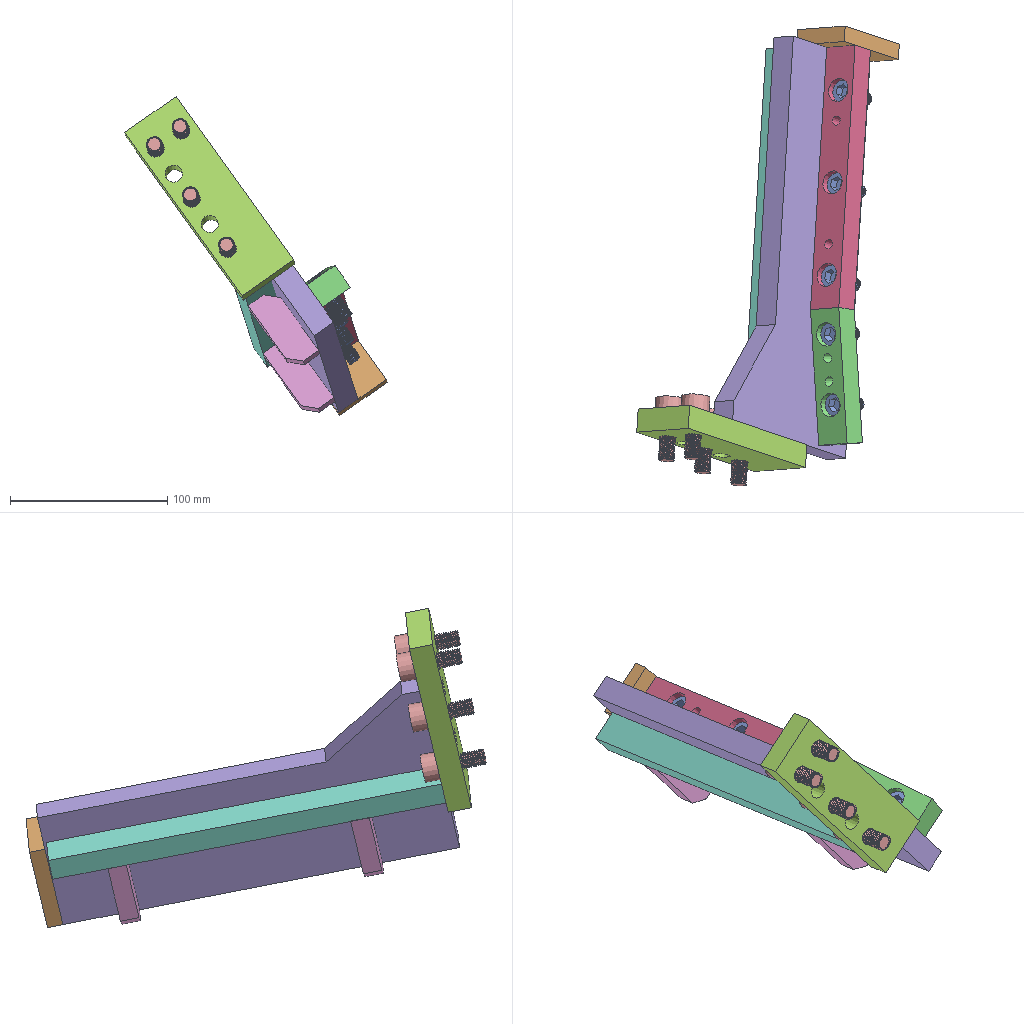Assembly | NX | 9 different items | 17 placed | box 167 x 292 x 203 mm
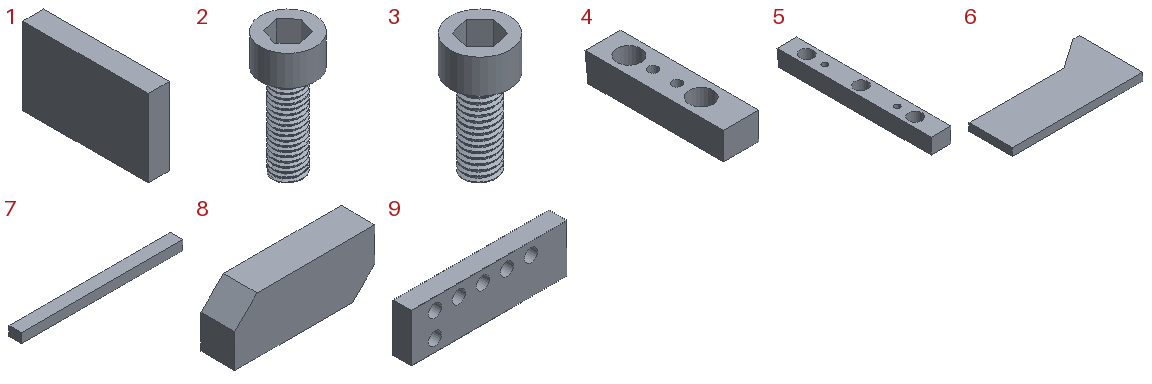Parts list (item | quantity | size | volume | features):
1 | x1 | 10 x 60 x 37 mm | 22200 mm3 | features DATUM_CSYS 2, EXTRUDE 1, SKETCH 1
2 | x4 | 18 x 18 x 40 mm | 3838 mm3 | features DATUM_CSYS 4, EXTRUDE 3, SKETCH 3, THREADS 1
3 | x5 | 14 x 14 x 28 mm | 1746 mm3 | features DATUM_CSYS 4, EXTRUDE 3, SKETCH 3, THREADS 1
4 | x1 | 22 x 86.4 x 17 mm | 26138 mm3 | features DATUM_CSYS 4, SKETCH 3, CBORE_HOLE 2, HOLE PACKAGE 2, SIMPLE HOLE 2, EXTRUDE 1
5 | x1 | 22 x 170.1 x 17 mm | 55003 mm3 | features DATUM_CSYS 4, CBORE_HOLE 3, SKETCH 3, HOLE PACKAGE 2, SIMPLE HOLE 2, EXTRUDE 1
6 | x1 | 257 x 125 x 15 mm | 352575 mm3 | features DATUM_CSYS 2, EXTRUDE 1, SKETCH 1
7 | x1 | 255 x 20 x 15 mm | 76500 mm3 | features DATUM_CSYS 2, EXTRUDE 1, SKETCH 1
8 | x2 | 50 x 12 x 20 mm | 11232 mm3 | features DATUM_CSYS 2, EXTRUDE 1, SKETCH 1
9 | x1 | 130 x 15 x 40 mm | 69447 mm3 | features DATUM_CSYS 2, EXTRUDE 1, SKETCH 1
Mates (type | each side: item.copy, entity, surface, feature):
Fix | 5.1 component | 2 times
Fix | 4.1 component
Touch | 8.1 edge | 6.1 edge
Touch | 7.1 edge | 6.1 edge
Touch | 8.1 face plane Extrude(1) | 6.1 face plane Extrude(1)